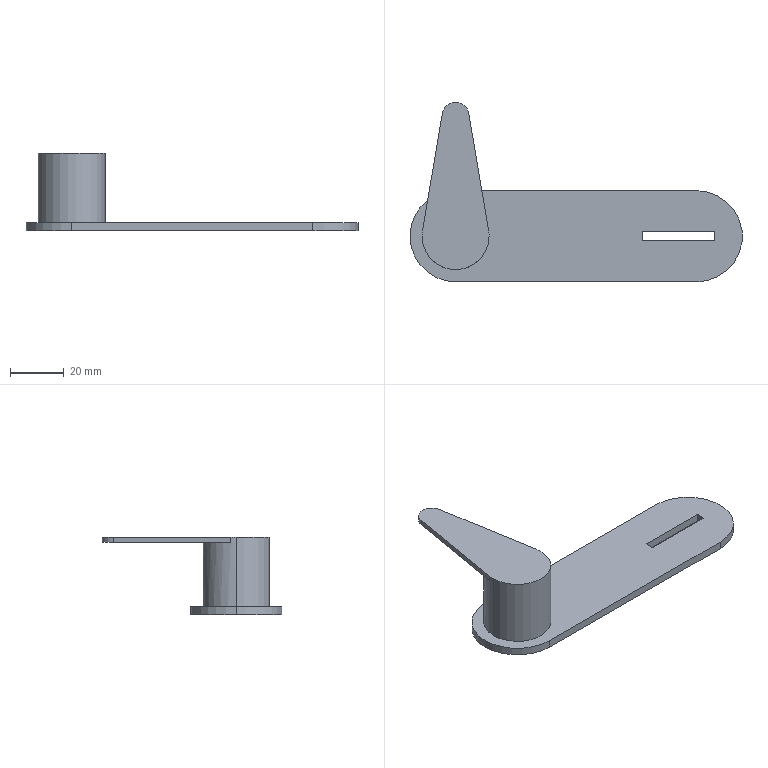Part | SolidWorks | features ICE 3, Extrusion 1 | 1 solid | 18 faces | box 124 x 67 x 29 mm | volume 25577 mm3 | plane 12 | cylinder 6 | commonest cylinder face diameters 34 x3 25 x2 10 x1
STEP:
#1=CARTESIAN_POINT('',(-32.5,0.,29.));
#2=VERTEX_POINT('',#1);
#3=CARTESIAN_POINT('',(-32.675,2.083,29.));
#4=VERTEX_POINT('',#3);
#5=CARTESIAN_POINT('',(-45.,0.,29.));
#6=DIRECTION('',(0.,0.,1.));
#7=DIRECTION('',(1.,0.,0.));
#8=AXIS2_PLACEMENT_3D('',#5,#6,#7);
#9=CIRCLE('',#8,12.5);
#10=EDGE_CURVE('',#2,#4,#9,.T.);
#11=ORIENTED_EDGE('',*,*,#10,.F.);
#12=CARTESIAN_POINT('',(-32.5,0.,3.));
#13=VERTEX_POINT('',#12);
#14=CARTESIAN_POINT('',(-32.5,0.,27.));
#15=DIRECTION('',(0.,0.,-1.));
#16=VECTOR('',#15,1000.);
#17=LINE('',#14,#16);
#18=EDGE_CURVE('',#2,#13,#17,.T.);
#19=ORIENTED_EDGE('',*,*,#18,.T.);
#20=CARTESIAN_POINT('',(-57.5,0.,3.));
#21=VERTEX_POINT('',#20);
#22=CARTESIAN_POINT('',(-45.,0.,3.));
#23=DIRECTION('',(0.,0.,1.));
#24=DIRECTION('',(1.,0.,0.));
#25=AXIS2_PLACEMENT_3D('',#22,#23,#24);
#26=CIRCLE('',#25,12.5);
#27=EDGE_CURVE('',#13,#21,#26,.T.);
#28=ORIENTED_EDGE('',*,*,#27,.T.);
#29=CARTESIAN_POINT('',(-57.5,0.,29.));
#30=VERTEX_POINT('',#29);
#31=CARTESIAN_POINT('',(-57.5,0.,27.));
#32=DIRECTION('',(0.,0.,-1.));
#33=VECTOR('',#32,1000.);
#34=LINE('',#31,#33);
#35=EDGE_CURVE('',#30,#21,#34,.T.);
#36=ORIENTED_EDGE('',*,*,#35,.F.);
#37=CARTESIAN_POINT('',(-57.325,2.083,29.));
#38=VERTEX_POINT('',#37);
#39=CARTESIAN_POINT('',(-45.,0.,29.));
#40=DIRECTION('',(0.,0.,1.));
#41=DIRECTION('',(1.,0.,0.));
#42=AXIS2_PLACEMENT_3D('',#39,#40,#41);
#43=CIRCLE('',#42,12.5);
#44=EDGE_CURVE('',#38,#30,#43,.T.);
#45=ORIENTED_EDGE('',*,*,#44,.F.);
#46=CARTESIAN_POINT('',(-57.325,2.083,27.));
#47=VERTEX_POINT('',#46);
#48=CARTESIAN_POINT('',(-57.325,2.083,29.));
#49=DIRECTION('',(0.,0.,-1.));
#50=VECTOR('',#49,1000.);
#51=LINE('',#48,#50);
#52=EDGE_CURVE('',#38,#47,#51,.T.);
#53=ORIENTED_EDGE('',*,*,#52,.T.);
#54=CARTESIAN_POINT('',(-32.675,2.083,27.));
#55=VERTEX_POINT('',#54);
#56=CARTESIAN_POINT('',(-45.,0.,27.));
#57=DIRECTION('',(0.,0.,1.));
#58=DIRECTION('',(1.,0.,0.));
#59=AXIS2_PLACEMENT_3D('',#56,#57,#58);
#60=CIRCLE('',#59,12.5);
#61=EDGE_CURVE('',#55,#47,#60,.T.);
#62=ORIENTED_EDGE('',*,*,#61,.F.);
#63=CARTESIAN_POINT('',(-32.675,2.083,29.));
#64=DIRECTION('',(0.,0.,-1.));
#65=VECTOR('',#64,1000.);
#66=LINE('',#63,#65);
#67=EDGE_CURVE('',#4,#55,#66,.T.);
#68=ORIENTED_EDGE('',*,*,#67,.F.);
#69=EDGE_LOOP('',(#11,#19,#28,#36,#45,#53,#62,#68));
#70=FACE_OUTER_BOUND('',#69,.T.);
#71=CARTESIAN_POINT('',(-45.,0.,27.));
#72=DIRECTION('',(0.,0.,-1.));
#73=DIRECTION('',(-1.,0.,0.));
#74=AXIS2_PLACEMENT_3D('',#71,#72,#73);
#75=CYLINDRICAL_SURFACE('',#74,12.5);
#76=ADVANCED_FACE('',(#70),#75,.T.);
#77=CARTESIAN_POINT('',(-62.,0.,3.));
#78=VERTEX_POINT('',#77);
#79=CARTESIAN_POINT('',(-45.,-17.,3.));
#80=VERTEX_POINT('',#79);
#81=CARTESIAN_POINT('',(-45.,0.,3.));
#82=DIRECTION('',(0.,0.,1.));
#83=DIRECTION('',(1.,0.,0.));
#84=AXIS2_PLACEMENT_3D('',#81,#82,#83);
#85=CIRCLE('',#84,17.);
#86=EDGE_CURVE('',#78,#80,#85,.T.);
#87=ORIENTED_EDGE('',*,*,#86,.F.);
#88=CARTESIAN_POINT('',(-62.,0.,0.));
#89=VERTEX_POINT('',#88);
#90=CARTESIAN_POINT('',(-62.,0.,3.));
#91=DIRECTION('',(0.,0.,-1.));
#92=VECTOR('',#91,1000.);
#93=LINE('',#90,#92);
#94=EDGE_CURVE('',#78,#89,#93,.T.);
#95=ORIENTED_EDGE('',*,*,#94,.T.);
#96=CARTESIAN_POINT('',(-45.,-17.,0.));
#97=VERTEX_POINT('',#96);
#98=CARTESIAN_POINT('',(-45.,0.,0.));
#99=DIRECTION('',(0.,0.,1.));
#100=DIRECTION('',(1.,0.,0.));
#101=AXIS2_PLACEMENT_3D('',#98,#99,#100);
#102=CIRCLE('',#101,17.);
#103=EDGE_CURVE('',#89,#97,#102,.T.);
#104=ORIENTED_EDGE('',*,*,#103,.T.);
#105=CARTESIAN_POINT('',(-45.,-17.,3.));
#106=DIRECTION('',(0.,0.,-1.));
#107=VECTOR('',#106,1000.);
#108=LINE('',#105,#107);
#109=EDGE_CURVE('',#80,#97,#108,.T.);
#110=ORIENTED_EDGE('',*,*,#109,.F.);
#111=EDGE_LOOP('',(#87,#95,#104,#110));
#112=FACE_OUTER_BOUND('',#111,.T.);
#113=CARTESIAN_POINT('',(-45.,0.,3.));
#114=DIRECTION('',(0.,0.,-1.));
#115=DIRECTION('',(-1.,0.,0.));
#116=AXIS2_PLACEMENT_3D('',#113,#114,#115);
#117=CYLINDRICAL_SURFACE('',#116,17.);
#118=ADVANCED_FACE('',(#112),#117,.T.);
#119=CARTESIAN_POINT('',(-45.,17.,3.));
#120=VERTEX_POINT('',#119);
#121=CARTESIAN_POINT('',(-45.,0.,3.));
#122=DIRECTION('',(0.,0.,1.));
#123=DIRECTION('',(1.,0.,0.));
#124=AXIS2_PLACEMENT_3D('',#121,#122,#123);
#125=CIRCLE('',#124,17.);
#126=EDGE_CURVE('',#120,#78,#125,.T.);
#127=ORIENTED_EDGE('',*,*,#126,.T.);
#128=ORIENTED_EDGE('',*,*,#86,.T.);
#129=CARTESIAN_POINT('',(45.,-17.,3.));
#130=VERTEX_POINT('',#129);
#131=CARTESIAN_POINT('',(-45.,-17.,3.));
#132=DIRECTION('',(1.,0.,0.));
#133=VECTOR('',#132,1000.);
#134=LINE('',#131,#133);
#135=EDGE_CURVE('',#80,#130,#134,.T.);
#136=ORIENTED_EDGE('',*,*,#135,.T.);
#137=CARTESIAN_POINT('',(45.,17.,3.));
#138=VERTEX_POINT('',#137);
#139=CARTESIAN_POINT('',(45.,0.,3.));
#140=DIRECTION('',(0.,0.,1.));
#141=DIRECTION('',(1.,0.,0.));
#142=AXIS2_PLACEMENT_3D('',#139,#140,#141);
#143=CIRCLE('',#142,17.);
#144=EDGE_CURVE('',#130,#138,#143,.T.);
#145=ORIENTED_EDGE('',*,*,#144,.T.);
#146=CARTESIAN_POINT('',(-45.,17.,3.));
#147=DIRECTION('',(-1.,0.,0.));
#148=VECTOR('',#147,1000.);
#149=LINE('',#146,#148);
#150=EDGE_CURVE('',#138,#120,#149,.T.);
#151=ORIENTED_EDGE('',*,*,#150,.T.);
#152=EDGE_LOOP('',(#127,#128,#136,#145,#151));
#153=FACE_OUTER_BOUND('',#152,.T.);
#154=CARTESIAN_POINT('',(24.637,-1.691,3.));
#155=VERTEX_POINT('',#154);
#156=CARTESIAN_POINT('',(24.637,1.691,3.));
#157=VERTEX_POINT('',#156);
#158=CARTESIAN_POINT('',(24.637,-1.691,3.));
#159=DIRECTION('',(0.,1.,0.));
#160=VECTOR('',#159,1000.);
#161=LINE('',#158,#160);
#162=EDGE_CURVE('',#155,#157,#161,.T.);
#163=ORIENTED_EDGE('',*,*,#162,.T.);
#164=CARTESIAN_POINT('',(51.69,1.691,3.));
#165=VERTEX_POINT('',#164);
#166=CARTESIAN_POINT('',(51.69,1.691,3.));
#167=DIRECTION('',(1.,0.,0.));
#168=VECTOR('',#167,1000.);
#169=LINE('',#166,#168);
#170=EDGE_CURVE('',#157,#165,#169,.T.);
#171=ORIENTED_EDGE('',*,*,#170,.T.);
#172=CARTESIAN_POINT('',(51.69,-1.691,3.));
#173=VERTEX_POINT('',#172);
#174=CARTESIAN_POINT('',(51.69,-1.691,3.));
#175=DIRECTION('',(0.,-1.,0.));
#176=VECTOR('',#175,1000.);
#177=LINE('',#174,#176);
#178=EDGE_CURVE('',#165,#173,#177,.T.);
#179=ORIENTED_EDGE('',*,*,#178,.T.);
#180=CARTESIAN_POINT('',(51.69,-1.691,3.));
#181=DIRECTION('',(-1.,0.,0.));
#182=VECTOR('',#181,1000.);
#183=LINE('',#180,#182);
#184=EDGE_CURVE('',#173,#155,#183,.T.);
#185=ORIENTED_EDGE('',*,*,#184,.T.);
#186=EDGE_LOOP('',(#163,#171,#179,#185));
#187=FACE_BOUND('',#186,.T.);
#188=CARTESIAN_POINT('',(-45.,0.,3.));
#189=DIRECTION('',(0.,0.,1.));
#190=DIRECTION('',(1.,0.,0.));
#191=AXIS2_PLACEMENT_3D('',#188,#189,#190);
#192=CIRCLE('',#191,12.5);
#193=EDGE_CURVE('',#21,#13,#192,.T.);
#194=ORIENTED_EDGE('',*,*,#193,.F.);
#195=ORIENTED_EDGE('',*,*,#27,.F.);
#196=EDGE_LOOP('',(#194,#195));
#197=FACE_BOUND('',#196,.T.);
#198=CARTESIAN_POINT('',(-45.,0.,3.));
#199=DIRECTION('',(0.,0.,1.));
#200=DIRECTION('',(1.,0.,0.));
#201=AXIS2_PLACEMENT_3D('',#198,#199,#200);
#202=PLANE('',#201);
#203=ADVANCED_FACE('',(#153,#187,#197),#202,.T.);
#204=ORIENTED_EDGE('',*,*,#94,.F.);
#205=ORIENTED_EDGE('',*,*,#126,.F.);
#206=CARTESIAN_POINT('',(-45.,17.,0.));
#207=VERTEX_POINT('',#206);
#208=CARTESIAN_POINT('',(-45.,17.,3.));
#209=DIRECTION('',(0.,0.,-1.));
#210=VECTOR('',#209,1000.);
#211=LINE('',#208,#210);
#212=EDGE_CURVE('',#120,#207,#211,.T.);
#213=ORIENTED_EDGE('',*,*,#212,.T.);
#214=CARTESIAN_POINT('',(-45.,0.,0.));
#215=DIRECTION('',(0.,0.,1.));
#216=DIRECTION('',(1.,0.,0.));
#217=AXIS2_PLACEMENT_3D('',#214,#215,#216);
#218=CIRCLE('',#217,17.);
#219=EDGE_CURVE('',#207,#89,#218,.T.);
#220=ORIENTED_EDGE('',*,*,#219,.T.);
#221=EDGE_LOOP('',(#204,#205,#213,#220));
#222=FACE_OUTER_BOUND('',#221,.T.);
#223=CARTESIAN_POINT('',(-45.,0.,3.));
#224=DIRECTION('',(0.,0.,-1.));
#225=DIRECTION('',(-1.,0.,0.));
#226=AXIS2_PLACEMENT_3D('',#223,#224,#225);
#227=CYLINDRICAL_SURFACE('',#226,17.);
#228=ADVANCED_FACE('',(#222),#227,.T.);
#229=CARTESIAN_POINT('',(45.,-17.,0.));
#230=VERTEX_POINT('',#229);
#231=CARTESIAN_POINT('',(-45.,-17.,0.));
#232=DIRECTION('',(1.,0.,0.));
#233=VECTOR('',#232,1000.);
#234=LINE('',#231,#233);
#235=EDGE_CURVE('',#97,#230,#234,.T.);
#236=ORIENTED_EDGE('',*,*,#235,.T.);
#237=CARTESIAN_POINT('',(45.,-17.,3.));
#238=DIRECTION('',(0.,0.,-1.));
#239=VECTOR('',#238,1000.);
#240=LINE('',#237,#239);
#241=EDGE_CURVE('',#130,#230,#240,.T.);
#242=ORIENTED_EDGE('',*,*,#241,.F.);
#243=ORIENTED_EDGE('',*,*,#135,.F.);
#244=ORIENTED_EDGE('',*,*,#109,.T.);
#245=EDGE_LOOP('',(#236,#242,#243,#244));
#246=FACE_OUTER_BOUND('',#245,.T.);
#247=CARTESIAN_POINT('',(-45.,-17.,3.));
#248=DIRECTION('',(0.,1.,0.));
#249=DIRECTION('',(0.,0.,1.));
#250=AXIS2_PLACEMENT_3D('',#247,#248,#249);
#251=PLANE('',#250);
#252=ADVANCED_FACE('',(#246),#251,.F.);
#253=CARTESIAN_POINT('',(45.,17.,0.));
#254=VERTEX_POINT('',#253);
#255=CARTESIAN_POINT('',(45.,0.,0.));
#256=DIRECTION('',(0.,0.,1.));
#257=DIRECTION('',(1.,0.,0.));
#258=AXIS2_PLACEMENT_3D('',#255,#256,#257);
#259=CIRCLE('',#258,17.);
#260=EDGE_CURVE('',#230,#254,#259,.T.);
#261=ORIENTED_EDGE('',*,*,#260,.T.);
#262=CARTESIAN_POINT('',(45.,17.,3.));
#263=DIRECTION('',(0.,0.,-1.));
#264=VECTOR('',#263,1000.);
#265=LINE('',#262,#264);
#266=EDGE_CURVE('',#138,#254,#265,.T.);
#267=ORIENTED_EDGE('',*,*,#266,.F.);
#268=ORIENTED_EDGE('',*,*,#144,.F.);
#269=ORIENTED_EDGE('',*,*,#241,.T.);
#270=EDGE_LOOP('',(#261,#267,#268,#269));
#271=FACE_OUTER_BOUND('',#270,.T.);
#272=CARTESIAN_POINT('',(45.,0.,3.));
#273=DIRECTION('',(0.,0.,-1.));
#274=DIRECTION('',(-1.,0.,0.));
#275=AXIS2_PLACEMENT_3D('',#272,#273,#274);
#276=CYLINDRICAL_SURFACE('',#275,17.);
#277=ADVANCED_FACE('',(#271),#276,.T.);
#278=CARTESIAN_POINT('',(-45.,17.,0.));
#279=DIRECTION('',(-1.,0.,0.));
#280=VECTOR('',#279,1000.);
#281=LINE('',#278,#280);
#282=EDGE_CURVE('',#254,#207,#281,.T.);
#283=ORIENTED_EDGE('',*,*,#282,.T.);
#284=ORIENTED_EDGE('',*,*,#212,.F.);
#285=ORIENTED_EDGE('',*,*,#150,.F.);
#286=ORIENTED_EDGE('',*,*,#266,.T.);
#287=EDGE_LOOP('',(#283,#284,#285,#286));
#288=FACE_OUTER_BOUND('',#287,.T.);
#289=CARTESIAN_POINT('',(-45.,17.,3.));
#290=DIRECTION('',(0.,-1.,0.));
#291=DIRECTION('',(1.,0.,0.));
#292=AXIS2_PLACEMENT_3D('',#289,#290,#291);
#293=PLANE('',#292);
#294=ADVANCED_FACE('',(#288),#293,.F.);
#295=CARTESIAN_POINT('',(24.637,1.691,0.));
#296=VERTEX_POINT('',#295);
#297=CARTESIAN_POINT('',(51.69,1.691,0.));
#298=VERTEX_POINT('',#297);
#299=CARTESIAN_POINT('',(51.69,1.691,0.));
#300=DIRECTION('',(1.,0.,0.));
#301=VECTOR('',#300,1000.);
#302=LINE('',#299,#301);
#303=EDGE_CURVE('',#296,#298,#302,.T.);
#304=ORIENTED_EDGE('',*,*,#303,.F.);
#305=CARTESIAN_POINT('',(24.637,-1.691,0.));
#306=VERTEX_POINT('',#305);
#307=CARTESIAN_POINT('',(24.637,-1.691,0.));
#308=DIRECTION('',(0.,1.,0.));
#309=VECTOR('',#308,1000.);
#310=LINE('',#307,#309);
#311=EDGE_CURVE('',#306,#296,#310,.T.);
#312=ORIENTED_EDGE('',*,*,#311,.F.);
#313=CARTESIAN_POINT('',(51.69,-1.691,0.));
#314=VERTEX_POINT('',#313);
#315=CARTESIAN_POINT('',(51.69,-1.691,0.));
#316=DIRECTION('',(-1.,0.,0.));
#317=VECTOR('',#316,1000.);
#318=LINE('',#315,#317);
#319=EDGE_CURVE('',#314,#306,#318,.T.);
#320=ORIENTED_EDGE('',*,*,#319,.F.);
#321=CARTESIAN_POINT('',(51.69,-1.691,0.));
#322=DIRECTION('',(0.,-1.,0.));
#323=VECTOR('',#322,1000.);
#324=LINE('',#321,#323);
#325=EDGE_CURVE('',#298,#314,#324,.T.);
#326=ORIENTED_EDGE('',*,*,#325,.F.);
#327=EDGE_LOOP('',(#304,#312,#320,#326));
#328=FACE_BOUND('',#327,.T.);
#329=ORIENTED_EDGE('',*,*,#219,.F.);
#330=ORIENTED_EDGE('',*,*,#282,.F.);
#331=ORIENTED_EDGE('',*,*,#260,.F.);
#332=ORIENTED_EDGE('',*,*,#235,.F.);
#333=ORIENTED_EDGE('',*,*,#103,.F.);
#334=EDGE_LOOP('',(#329,#330,#331,#332,#333));
#335=FACE_OUTER_BOUND('',#334,.T.);
#336=CARTESIAN_POINT('',(-45.,0.,0.));
#337=DIRECTION('',(0.,0.,1.));
#338=DIRECTION('',(1.,0.,0.));
#339=AXIS2_PLACEMENT_3D('',#336,#337,#338);
#340=PLANE('',#339);
#341=ADVANCED_FACE('',(#328,#335),#340,.F.);
#342=ORIENTED_EDGE('',*,*,#311,.T.);
#343=CARTESIAN_POINT('',(24.637,1.691,3.));
#344=DIRECTION('',(0.,0.,-1.));
#345=VECTOR('',#344,1000.);
#346=LINE('',#343,#345);
#347=EDGE_CURVE('',#157,#296,#346,.T.);
#348=ORIENTED_EDGE('',*,*,#347,.F.);
#349=ORIENTED_EDGE('',*,*,#162,.F.);
#350=CARTESIAN_POINT('',(24.637,-1.691,3.));
#351=DIRECTION('',(0.,0.,-1.));
#352=VECTOR('',#351,1000.);
#353=LINE('',#350,#352);
#354=EDGE_CURVE('',#155,#306,#353,.T.);
#355=ORIENTED_EDGE('',*,*,#354,.T.);
#356=EDGE_LOOP('',(#342,#348,#349,#355));
#357=FACE_OUTER_BOUND('',#356,.T.);
#358=CARTESIAN_POINT('',(24.637,-1.691,3.));
#359=DIRECTION('',(-1.,0.,0.));
#360=DIRECTION('',(0.,0.,1.));
#361=AXIS2_PLACEMENT_3D('',#358,#359,#360);
#362=PLANE('',#361);
#363=ADVANCED_FACE('',(#357),#362,.F.);
#364=ORIENTED_EDGE('',*,*,#319,.T.);
#365=ORIENTED_EDGE('',*,*,#354,.F.);
#366=ORIENTED_EDGE('',*,*,#184,.F.);
#367=CARTESIAN_POINT('',(51.69,-1.691,3.));
#368=DIRECTION('',(0.,0.,-1.));
#369=VECTOR('',#368,1000.);
#370=LINE('',#367,#369);
#371=EDGE_CURVE('',#173,#314,#370,.T.);
#372=ORIENTED_EDGE('',*,*,#371,.T.);
#373=EDGE_LOOP('',(#364,#365,#366,#372));
#374=FACE_OUTER_BOUND('',#373,.T.);
#375=CARTESIAN_POINT('',(51.69,-1.691,3.));
#376=DIRECTION('',(0.,-1.,0.));
#377=DIRECTION('',(0.,0.,-1.));
#378=AXIS2_PLACEMENT_3D('',#375,#376,#377);
#379=PLANE('',#378);
#380=ADVANCED_FACE('',(#374),#379,.F.);
#381=ORIENTED_EDGE('',*,*,#325,.T.);
#382=ORIENTED_EDGE('',*,*,#371,.F.);
#383=ORIENTED_EDGE('',*,*,#178,.F.);
#384=CARTESIAN_POINT('',(51.69,1.691,3.));
#385=DIRECTION('',(0.,0.,-1.));
#386=VECTOR('',#385,1000.);
#387=LINE('',#384,#386);
#388=EDGE_CURVE('',#165,#298,#387,.T.);
#389=ORIENTED_EDGE('',*,*,#388,.T.);
#390=EDGE_LOOP('',(#381,#382,#383,#389));
#391=FACE_OUTER_BOUND('',#390,.T.);
#392=CARTESIAN_POINT('',(51.69,-1.691,3.));
#393=DIRECTION('',(1.,0.,0.));
#394=DIRECTION('',(0.,0.,-1.));
#395=AXIS2_PLACEMENT_3D('',#392,#393,#394);
#396=PLANE('',#395);
#397=ADVANCED_FACE('',(#391),#396,.F.);
#398=ORIENTED_EDGE('',*,*,#303,.T.);
#399=ORIENTED_EDGE('',*,*,#388,.F.);
#400=ORIENTED_EDGE('',*,*,#170,.F.);
#401=ORIENTED_EDGE('',*,*,#347,.T.);
#402=EDGE_LOOP('',(#398,#399,#400,#401));
#403=FACE_OUTER_BOUND('',#402,.T.);
#404=CARTESIAN_POINT('',(51.69,1.691,3.));
#405=DIRECTION('',(0.,1.,0.));
#406=DIRECTION('',(0.,0.,1.));
#407=AXIS2_PLACEMENT_3D('',#404,#405,#406);
#408=PLANE('',#407);
#409=ADVANCED_FACE('',(#403),#408,.F.);
#410=ORIENTED_EDGE('',*,*,#18,.F.);
#411=CARTESIAN_POINT('',(-45.,0.,29.));
#412=DIRECTION('',(0.,0.,1.));
#413=DIRECTION('',(1.,0.,0.));
#414=AXIS2_PLACEMENT_3D('',#411,#412,#413);
#415=CIRCLE('',#414,12.5);
#416=EDGE_CURVE('',#30,#2,#415,.T.);
#417=ORIENTED_EDGE('',*,*,#416,.F.);
#418=ORIENTED_EDGE('',*,*,#35,.T.);
#419=ORIENTED_EDGE('',*,*,#193,.T.);
#420=EDGE_LOOP('',(#410,#417,#418,#419));
#421=FACE_OUTER_BOUND('',#420,.T.);
#422=CARTESIAN_POINT('',(-45.,0.,27.));
#423=DIRECTION('',(0.,0.,-1.));
#424=DIRECTION('',(-1.,0.,0.));
#425=AXIS2_PLACEMENT_3D('',#422,#423,#424);
#426=CYLINDRICAL_SURFACE('',#425,12.5);
#427=ADVANCED_FACE('',(#421),#426,.T.);
#428=CARTESIAN_POINT('',(-40.07,45.833,27.));
#429=VERTEX_POINT('',#428);
#430=CARTESIAN_POINT('',(-40.07,45.833,27.));
#431=DIRECTION('',(-0.1667,0.986,0.));
#432=VECTOR('',#431,1000.);
#433=LINE('',#430,#432);
#434=EDGE_CURVE('',#55,#429,#433,.T.);
#435=ORIENTED_EDGE('',*,*,#434,.F.);
#436=ORIENTED_EDGE('',*,*,#61,.T.);
#437=CARTESIAN_POINT('',(-49.93,45.833,27.));
#438=VERTEX_POINT('',#437);
#439=CARTESIAN_POINT('',(-57.325,2.083,27.));
#440=DIRECTION('',(-0.1667,-0.986,0.));
#441=VECTOR('',#440,1000.);
#442=LINE('',#439,#441);
#443=EDGE_CURVE('',#438,#47,#442,.T.);
#444=ORIENTED_EDGE('',*,*,#443,.F.);
#445=CARTESIAN_POINT('',(-45.,45.,27.));
#446=DIRECTION('',(0.,0.,1.));
#447=DIRECTION('',(1.,0.,0.));
#448=AXIS2_PLACEMENT_3D('',#445,#446,#447);
#449=CIRCLE('',#448,5.);
#450=EDGE_CURVE('',#429,#438,#449,.T.);
#451=ORIENTED_EDGE('',*,*,#450,.F.);
#452=EDGE_LOOP('',(#435,#436,#444,#451));
#453=FACE_OUTER_BOUND('',#452,.T.);
#454=CARTESIAN_POINT('',(-45.,0.,27.));
#455=DIRECTION('',(0.,0.,1.));
#456=DIRECTION('',(1.,0.,0.));
#457=AXIS2_PLACEMENT_3D('',#454,#455,#456);
#458=PLANE('',#457);
#459=ADVANCED_FACE('',(#453),#458,.F.);
#460=ORIENTED_EDGE('',*,*,#434,.T.);
#461=CARTESIAN_POINT('',(-40.07,45.833,29.));
#462=VERTEX_POINT('',#461);
#463=CARTESIAN_POINT('',(-40.07,45.833,29.));
#464=DIRECTION('',(0.,0.,-1.));
#465=VECTOR('',#464,1000.);
#466=LINE('',#463,#465);
#467=EDGE_CURVE('',#462,#429,#466,.T.);
#468=ORIENTED_EDGE('',*,*,#467,.F.);
#469=CARTESIAN_POINT('',(-40.07,45.833,29.));
#470=DIRECTION('',(-0.1667,0.986,0.));
#471=VECTOR('',#470,1000.);
#472=LINE('',#469,#471);
#473=EDGE_CURVE('',#4,#462,#472,.T.);
#474=ORIENTED_EDGE('',*,*,#473,.F.);
#475=ORIENTED_EDGE('',*,*,#67,.T.);
#476=EDGE_LOOP('',(#460,#468,#474,#475));
#477=FACE_OUTER_BOUND('',#476,.T.);
#478=CARTESIAN_POINT('',(-40.07,45.833,29.));
#479=DIRECTION('',(-0.986,-0.1667,0.));
#480=DIRECTION('',(0.1667,-0.986,0.));
#481=AXIS2_PLACEMENT_3D('',#478,#479,#480);
#482=PLANE('',#481);
#483=ADVANCED_FACE('',(#477),#482,.F.);
#484=ORIENTED_EDGE('',*,*,#450,.T.);
#485=CARTESIAN_POINT('',(-49.93,45.833,29.));
#486=VERTEX_POINT('',#485);
#487=CARTESIAN_POINT('',(-49.93,45.833,29.));
#488=DIRECTION('',(0.,0.,-1.));
#489=VECTOR('',#488,1000.);
#490=LINE('',#487,#489);
#491=EDGE_CURVE('',#486,#438,#490,.T.);
#492=ORIENTED_EDGE('',*,*,#491,.F.);
#493=CARTESIAN_POINT('',(-45.,45.,29.));
#494=DIRECTION('',(0.,0.,1.));
#495=DIRECTION('',(1.,0.,0.));
#496=AXIS2_PLACEMENT_3D('',#493,#494,#495);
#497=CIRCLE('',#496,5.);
#498=EDGE_CURVE('',#462,#486,#497,.T.);
#499=ORIENTED_EDGE('',*,*,#498,.F.);
#500=ORIENTED_EDGE('',*,*,#467,.T.);
#501=EDGE_LOOP('',(#484,#492,#499,#500));
#502=FACE_OUTER_BOUND('',#501,.T.);
#503=CARTESIAN_POINT('',(-45.,45.,29.));
#504=DIRECTION('',(0.,0.,-1.));
#505=DIRECTION('',(-1.,0.,0.));
#506=AXIS2_PLACEMENT_3D('',#503,#504,#505);
#507=CYLINDRICAL_SURFACE('',#506,5.);
#508=ADVANCED_FACE('',(#502),#507,.T.);
#509=ORIENTED_EDGE('',*,*,#443,.T.);
#510=ORIENTED_EDGE('',*,*,#52,.F.);
#511=CARTESIAN_POINT('',(-57.325,2.083,29.));
#512=DIRECTION('',(-0.1667,-0.986,0.));
#513=VECTOR('',#512,1000.);
#514=LINE('',#511,#513);
#515=EDGE_CURVE('',#486,#38,#514,.T.);
#516=ORIENTED_EDGE('',*,*,#515,.F.);
#517=ORIENTED_EDGE('',*,*,#491,.T.);
#518=EDGE_LOOP('',(#509,#510,#516,#517));
#519=FACE_OUTER_BOUND('',#518,.T.);
#520=CARTESIAN_POINT('',(-57.325,2.083,29.));
#521=DIRECTION('',(0.986,-0.1667,0.));
#522=DIRECTION('',(0.1667,0.986,0.));
#523=AXIS2_PLACEMENT_3D('',#520,#521,#522);
#524=PLANE('',#523);
#525=ADVANCED_FACE('',(#519),#524,.F.);
#526=ORIENTED_EDGE('',*,*,#44,.T.);
#527=ORIENTED_EDGE('',*,*,#416,.T.);
#528=ORIENTED_EDGE('',*,*,#10,.T.);
#529=ORIENTED_EDGE('',*,*,#473,.T.);
#530=ORIENTED_EDGE('',*,*,#498,.T.);
#531=ORIENTED_EDGE('',*,*,#515,.T.);
#532=EDGE_LOOP('',(#526,#527,#528,#529,#530,#531));
#533=FACE_OUTER_BOUND('',#532,.T.);
#534=CARTESIAN_POINT('',(-45.,0.,29.));
#535=DIRECTION('',(0.,0.,1.));
#536=DIRECTION('',(1.,0.,0.));
#537=AXIS2_PLACEMENT_3D('',#534,#535,#536);
#538=PLANE('',#537);
#539=ADVANCED_FACE('',(#533),#538,.T.);
#540=CLOSED_SHELL('',(#76,#118,#203,#228,#252,#277,#294,#341,#363,#380,#397,#409,#427,#459,#483,#508,#525,#539));
#541=MANIFOLD_SOLID_BREP('',#540);
#542=CARTESIAN_POINT('',(0.,0.,0.));
#543=DIRECTION('',(0.,0.,1.));
#544=DIRECTION('',(1.,0.,0.));
#545=AXIS2_PLACEMENT_3D('',#542,#543,#544);
#546=(LENGTH_UNIT()NAMED_UNIT(*)SI_UNIT(.MILLI.,.METRE.));
#547=UNCERTAINTY_MEASURE_WITH_UNIT(LENGTH_MEASURE(0.00001),#546,'','');
#548=(NAMED_UNIT(*)PLANE_ANGLE_UNIT()SI_UNIT($,.RADIAN.));
#549=(NAMED_UNIT(*)SI_UNIT($,.STERADIAN.)SOLID_ANGLE_UNIT());
#550=(GEOMETRIC_REPRESENTATION_CONTEXT(3)GLOBAL_UNCERTAINTY_ASSIGNED_CONTEXT((#547))GLOBAL_UNIT_ASSIGNED_CONTEXT((#546,#548,#549))REPRESENTATION_CONTEXT('',''));
#551=ADVANCED_BREP_SHAPE_REPRESENTATION('',(#541,#545),#550);